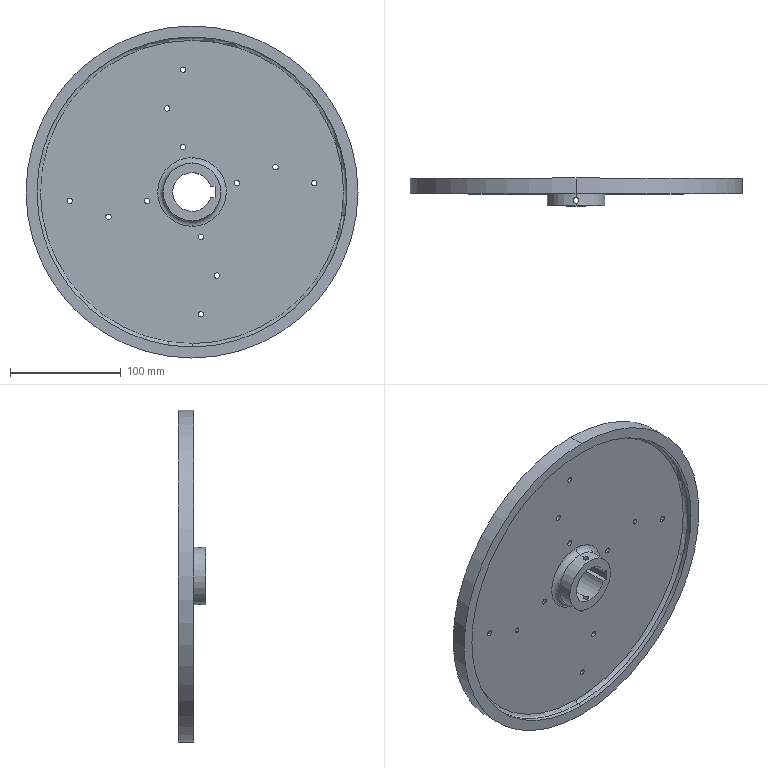Part | NX | features BREP 1 | 1 solid | 48 faces | box 300 x 25 x 300 mm | volume 572533 mm3 | cylinder 37 | plane 7 | torus 4 | commonest cylinder face diameters 4.917 x24 5 x4 35 x3 52 x2 280 x2 300 x2